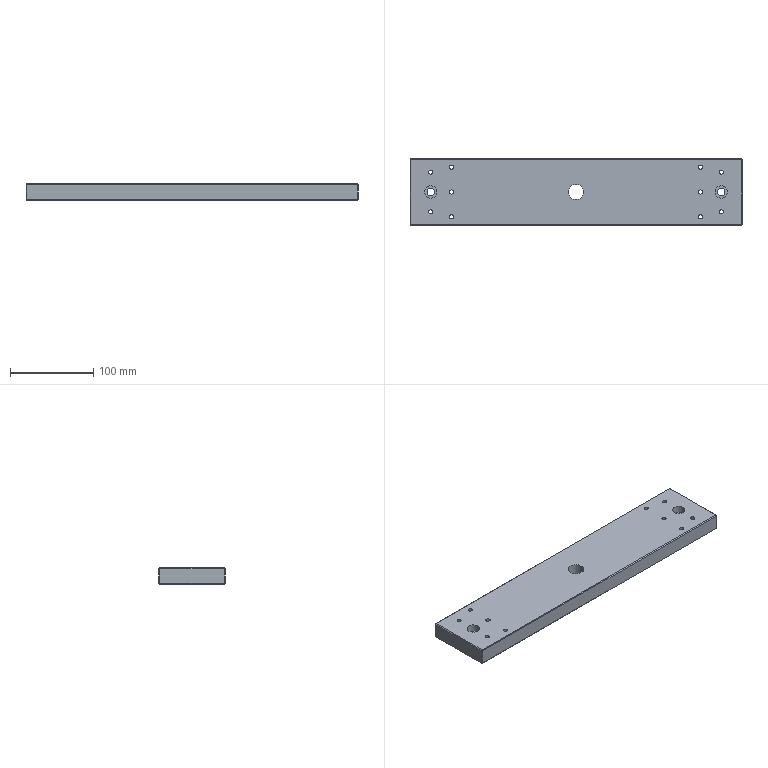Part | STEP file | Hold-down fixture fixing plate | 1 solid | 58 faces | box 400 x 80 x 20 mm | volume 625122 mm3 | cylinder 30 | plane 28 | commonest cylinder face diameters 5 x20 9 x4 15 x4 18.5 x2